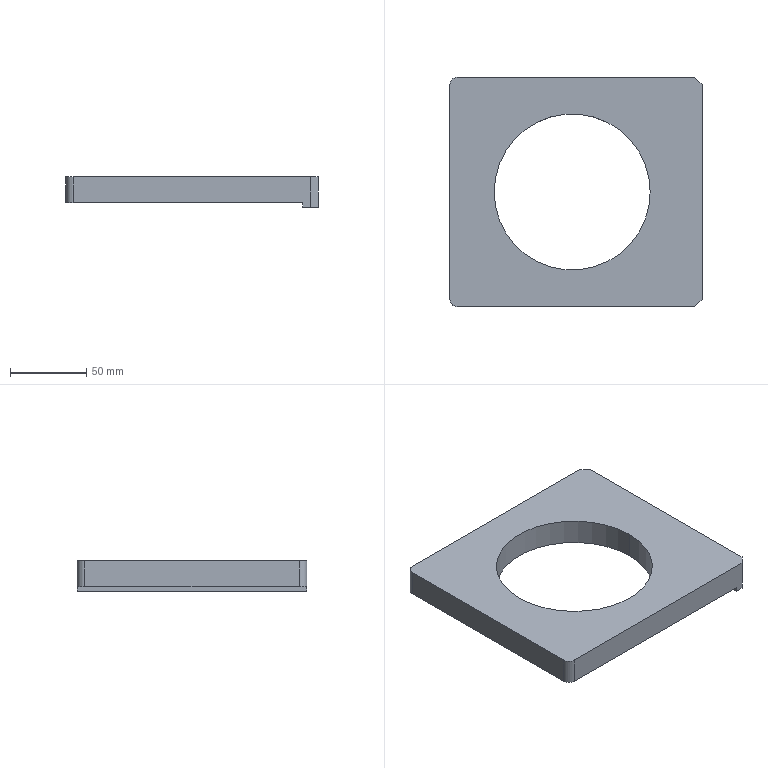Part | SolidWorks | features BaseBody 1 | 1 solid | 14 faces | box 165 x 150 x 20 mm | volume 285656 mm3 | plane 10 | cylinder 4 | commonest cylinder face diameters 10 x2 102 x2
STEP:
#1=CARTESIAN_POINT('',(-51.,0.,20.));
#2=VERTEX_POINT('',#1);
#3=CARTESIAN_POINT('',(51.,0.,20.));
#4=VERTEX_POINT('',#3);
#5=CARTESIAN_POINT('',(0.,0.,20.));
#6=DIRECTION('',(0.,0.,1.));
#7=DIRECTION('',(1.,0.,0.));
#8=AXIS2_PLACEMENT_3D('',#5,#6,#7);
#9=CIRCLE('',#8,51.);
#10=EDGE_CURVE('',#2,#4,#9,.T.);
#11=ORIENTED_EDGE('',*,*,#10,.T.);
#12=CARTESIAN_POINT('',(51.,0.,3.));
#13=VERTEX_POINT('',#12);
#14=CARTESIAN_POINT('',(51.,0.,20.));
#15=DIRECTION('',(0.,0.,-1.));
#16=VECTOR('',#15,1000.);
#17=LINE('',#14,#16);
#18=EDGE_CURVE('',#4,#13,#17,.T.);
#19=ORIENTED_EDGE('',*,*,#18,.T.);
#20=CARTESIAN_POINT('',(-51.,0.,3.));
#21=VERTEX_POINT('',#20);
#22=CARTESIAN_POINT('',(0.,0.,3.));
#23=DIRECTION('',(0.,0.,-1.));
#24=DIRECTION('',(-1.,0.,0.));
#25=AXIS2_PLACEMENT_3D('',#22,#23,#24);
#26=CIRCLE('',#25,51.);
#27=EDGE_CURVE('',#13,#21,#26,.T.);
#28=ORIENTED_EDGE('',*,*,#27,.T.);
#29=CARTESIAN_POINT('',(-51.,0.,20.));
#30=DIRECTION('',(0.,0.,-1.));
#31=VECTOR('',#30,1000.);
#32=LINE('',#29,#31);
#33=EDGE_CURVE('',#2,#21,#32,.T.);
#34=ORIENTED_EDGE('',*,*,#33,.F.);
#35=EDGE_LOOP('',(#11,#19,#28,#34));
#36=FACE_OUTER_BOUND('',#35,.T.);
#37=CARTESIAN_POINT('',(0.,0.,20.));
#38=DIRECTION('',(0.,0.,-1.));
#39=DIRECTION('',(-1.,0.,0.));
#40=AXIS2_PLACEMENT_3D('',#37,#38,#39);
#41=CYLINDRICAL_SURFACE('',#40,51.);
#42=ADVANCED_FACE('',(#36),#41,.F.);
#43=ORIENTED_EDGE('',*,*,#10,.F.);
#44=CARTESIAN_POINT('',(0.,0.,20.));
#45=DIRECTION('',(0.,0.,1.));
#46=DIRECTION('',(1.,0.,0.));
#47=AXIS2_PLACEMENT_3D('',#44,#45,#46);
#48=CIRCLE('',#47,51.);
#49=EDGE_CURVE('',#4,#2,#48,.T.);
#50=ORIENTED_EDGE('',*,*,#49,.F.);
#51=EDGE_LOOP('',(#43,#50));
#52=FACE_BOUND('',#51,.T.);
#53=CARTESIAN_POINT('',(-80.,-70.,20.));
#54=VERTEX_POINT('',#53);
#55=CARTESIAN_POINT('',(-75.,-75.,20.));
#56=VERTEX_POINT('',#55);
#57=CARTESIAN_POINT('',(-75.,-70.,20.));
#58=DIRECTION('',(0.,0.,1.));
#59=DIRECTION('',(1.,0.,0.));
#60=AXIS2_PLACEMENT_3D('',#57,#58,#59);
#61=CIRCLE('',#60,5.);
#62=EDGE_CURVE('',#54,#56,#61,.T.);
#63=ORIENTED_EDGE('',*,*,#62,.T.);
#64=CARTESIAN_POINT('',(80.,-75.,20.));
#65=VERTEX_POINT('',#64);
#66=CARTESIAN_POINT('',(0.,-75.,20.));
#67=DIRECTION('',(1.,0.,0.));
#68=VECTOR('',#67,1000.);
#69=LINE('',#66,#68);
#70=EDGE_CURVE('',#56,#65,#69,.T.);
#71=ORIENTED_EDGE('',*,*,#70,.T.);
#72=CARTESIAN_POINT('',(85.,-70.,20.));
#73=VERTEX_POINT('',#72);
#74=CARTESIAN_POINT('',(77.5,-77.5,20.));
#75=DIRECTION('',(0.7071,0.7071,0.));
#76=VECTOR('',#75,1000.);
#77=LINE('',#74,#76);
#78=EDGE_CURVE('',#65,#73,#77,.T.);
#79=ORIENTED_EDGE('',*,*,#78,.T.);
#80=CARTESIAN_POINT('',(85.,70.,20.));
#81=VERTEX_POINT('',#80);
#82=CARTESIAN_POINT('',(85.,80.,20.));
#83=DIRECTION('',(0.,1.,0.));
#84=VECTOR('',#83,1000.);
#85=LINE('',#82,#84);
#86=EDGE_CURVE('',#73,#81,#85,.T.);
#87=ORIENTED_EDGE('',*,*,#86,.T.);
#88=CARTESIAN_POINT('',(80.,75.,20.));
#89=VERTEX_POINT('',#88);
#90=CARTESIAN_POINT('',(77.5,77.5,20.));
#91=DIRECTION('',(-0.7071,0.7071,0.));
#92=VECTOR('',#91,1000.);
#93=LINE('',#90,#92);
#94=EDGE_CURVE('',#81,#89,#93,.T.);
#95=ORIENTED_EDGE('',*,*,#94,.T.);
#96=CARTESIAN_POINT('',(-75.,75.,20.));
#97=VERTEX_POINT('',#96);
#98=CARTESIAN_POINT('',(0.,75.,20.));
#99=DIRECTION('',(-1.,0.,0.));
#100=VECTOR('',#99,1000.);
#101=LINE('',#98,#100);
#102=EDGE_CURVE('',#89,#97,#101,.T.);
#103=ORIENTED_EDGE('',*,*,#102,.T.);
#104=CARTESIAN_POINT('',(-80.,70.,20.));
#105=VERTEX_POINT('',#104);
#106=CARTESIAN_POINT('',(-75.,70.,20.));
#107=DIRECTION('',(0.,0.,1.));
#108=DIRECTION('',(1.,0.,0.));
#109=AXIS2_PLACEMENT_3D('',#106,#107,#108);
#110=CIRCLE('',#109,5.);
#111=EDGE_CURVE('',#97,#105,#110,.T.);
#112=ORIENTED_EDGE('',*,*,#111,.T.);
#113=CARTESIAN_POINT('',(-80.,0.,20.));
#114=DIRECTION('',(0.,-1.,0.));
#115=VECTOR('',#114,1000.);
#116=LINE('',#113,#115);
#117=EDGE_CURVE('',#105,#54,#116,.T.);
#118=ORIENTED_EDGE('',*,*,#117,.T.);
#119=EDGE_LOOP('',(#63,#71,#79,#87,#95,#103,#112,#118));
#120=FACE_OUTER_BOUND('',#119,.T.);
#121=CARTESIAN_POINT('',(0.,0.,20.));
#122=DIRECTION('',(0.,0.,1.));
#123=DIRECTION('',(1.,0.,0.));
#124=AXIS2_PLACEMENT_3D('',#121,#122,#123);
#125=PLANE('',#124);
#126=ADVANCED_FACE('',(#52,#120),#125,.T.);
#127=CARTESIAN_POINT('',(75.,-75.,0.));
#128=VERTEX_POINT('',#127);
#129=CARTESIAN_POINT('',(80.,-75.,0.));
#130=VERTEX_POINT('',#129);
#131=CARTESIAN_POINT('',(0.,-75.,0.));
#132=DIRECTION('',(1.,0.,0.));
#133=VECTOR('',#132,1000.);
#134=LINE('',#131,#133);
#135=EDGE_CURVE('',#128,#130,#134,.T.);
#136=ORIENTED_EDGE('',*,*,#135,.F.);
#137=CARTESIAN_POINT('',(75.,75.,0.));
#138=VERTEX_POINT('',#137);
#139=CARTESIAN_POINT('',(75.,-80.,0.));
#140=DIRECTION('',(0.,-1.,0.));
#141=VECTOR('',#140,1000.);
#142=LINE('',#139,#141);
#143=EDGE_CURVE('',#138,#128,#142,.T.);
#144=ORIENTED_EDGE('',*,*,#143,.F.);
#145=CARTESIAN_POINT('',(80.,75.,0.));
#146=VERTEX_POINT('',#145);
#147=CARTESIAN_POINT('',(0.,75.,0.));
#148=DIRECTION('',(-1.,0.,0.));
#149=VECTOR('',#148,1000.);
#150=LINE('',#147,#149);
#151=EDGE_CURVE('',#146,#138,#150,.T.);
#152=ORIENTED_EDGE('',*,*,#151,.F.);
#153=CARTESIAN_POINT('',(85.,70.,0.));
#154=VERTEX_POINT('',#153);
#155=CARTESIAN_POINT('',(75.,80.,0.));
#156=DIRECTION('',(0.7071,-0.7071,0.));
#157=VECTOR('',#156,1000.);
#158=LINE('',#155,#157);
#159=EDGE_CURVE('',#146,#154,#158,.T.);
#160=ORIENTED_EDGE('',*,*,#159,.T.);
#161=CARTESIAN_POINT('',(85.,-70.,0.));
#162=VERTEX_POINT('',#161);
#163=CARTESIAN_POINT('',(85.,80.,0.));
#164=DIRECTION('',(0.,1.,0.));
#165=VECTOR('',#164,1000.);
#166=LINE('',#163,#165);
#167=EDGE_CURVE('',#162,#154,#166,.T.);
#168=ORIENTED_EDGE('',*,*,#167,.F.);
#169=CARTESIAN_POINT('',(85.,-70.,0.));
#170=DIRECTION('',(-0.7071,-0.7071,0.));
#171=VECTOR('',#170,1000.);
#172=LINE('',#169,#171);
#173=EDGE_CURVE('',#162,#130,#172,.T.);
#174=ORIENTED_EDGE('',*,*,#173,.T.);
#175=EDGE_LOOP('',(#136,#144,#152,#160,#168,#174));
#176=FACE_OUTER_BOUND('',#175,.T.);
#177=CARTESIAN_POINT('',(0.,0.,0.));
#178=DIRECTION('',(0.,0.,1.));
#179=DIRECTION('',(1.,0.,0.));
#180=AXIS2_PLACEMENT_3D('',#177,#178,#179);
#181=PLANE('',#180);
#182=ADVANCED_FACE('',(#176),#181,.F.);
#183=ORIENTED_EDGE('',*,*,#78,.F.);
#184=CARTESIAN_POINT('',(80.,-75.,20.));
#185=DIRECTION('',(0.,0.,-1.));
#186=VECTOR('',#185,1000.);
#187=LINE('',#184,#186);
#188=EDGE_CURVE('',#65,#130,#187,.T.);
#189=ORIENTED_EDGE('',*,*,#188,.T.);
#190=ORIENTED_EDGE('',*,*,#173,.F.);
#191=CARTESIAN_POINT('',(85.,-70.,20.));
#192=DIRECTION('',(0.,0.,-1.));
#193=VECTOR('',#192,1000.);
#194=LINE('',#191,#193);
#195=EDGE_CURVE('',#73,#162,#194,.T.);
#196=ORIENTED_EDGE('',*,*,#195,.F.);
#197=EDGE_LOOP('',(#183,#189,#190,#196));
#198=FACE_OUTER_BOUND('',#197,.T.);
#199=CARTESIAN_POINT('',(85.,-70.,20.));
#200=DIRECTION('',(-0.7071,0.7071,0.));
#201=DIRECTION('',(0.,0.,-1.));
#202=AXIS2_PLACEMENT_3D('',#199,#200,#201);
#203=PLANE('',#202);
#204=ADVANCED_FACE('',(#198),#203,.F.);
#205=ORIENTED_EDGE('',*,*,#159,.F.);
#206=CARTESIAN_POINT('',(80.,75.,20.));
#207=DIRECTION('',(0.,0.,1.));
#208=VECTOR('',#207,1000.);
#209=LINE('',#206,#208);
#210=EDGE_CURVE('',#146,#89,#209,.T.);
#211=ORIENTED_EDGE('',*,*,#210,.T.);
#212=ORIENTED_EDGE('',*,*,#94,.F.);
#213=CARTESIAN_POINT('',(85.,70.,20.));
#214=DIRECTION('',(0.,0.,1.));
#215=VECTOR('',#214,1000.);
#216=LINE('',#213,#215);
#217=EDGE_CURVE('',#154,#81,#216,.T.);
#218=ORIENTED_EDGE('',*,*,#217,.F.);
#219=EDGE_LOOP('',(#205,#211,#212,#218));
#220=FACE_OUTER_BOUND('',#219,.T.);
#221=CARTESIAN_POINT('',(75.,80.,20.));
#222=DIRECTION('',(-0.7071,-0.7071,0.));
#223=DIRECTION('',(0.,0.,-1.));
#224=AXIS2_PLACEMENT_3D('',#221,#222,#223);
#225=PLANE('',#224);
#226=ADVANCED_FACE('',(#220),#225,.F.);
#227=CARTESIAN_POINT('',(75.,-75.,3.));
#228=VERTEX_POINT('',#227);
#229=CARTESIAN_POINT('',(75.,-75.,3.));
#230=DIRECTION('',(0.,0.,-1.));
#231=VECTOR('',#230,1000.);
#232=LINE('',#229,#231);
#233=EDGE_CURVE('',#228,#128,#232,.T.);
#234=ORIENTED_EDGE('',*,*,#233,.F.);
#235=CARTESIAN_POINT('',(75.,75.,3.));
#236=VERTEX_POINT('',#235);
#237=CARTESIAN_POINT('',(75.,-80.,3.));
#238=DIRECTION('',(0.,-1.,0.));
#239=VECTOR('',#238,1000.);
#240=LINE('',#237,#239);
#241=EDGE_CURVE('',#236,#228,#240,.T.);
#242=ORIENTED_EDGE('',*,*,#241,.F.);
#243=CARTESIAN_POINT('',(75.,75.,3.));
#244=DIRECTION('',(0.,0.,1.));
#245=VECTOR('',#244,1000.);
#246=LINE('',#243,#245);
#247=EDGE_CURVE('',#138,#236,#246,.T.);
#248=ORIENTED_EDGE('',*,*,#247,.F.);
#249=ORIENTED_EDGE('',*,*,#143,.T.);
#250=EDGE_LOOP('',(#234,#242,#248,#249));
#251=FACE_OUTER_BOUND('',#250,.T.);
#252=CARTESIAN_POINT('',(75.,-80.,3.));
#253=DIRECTION('',(1.,0.,0.));
#254=DIRECTION('',(0.,0.,1.));
#255=AXIS2_PLACEMENT_3D('',#252,#253,#254);
#256=PLANE('',#255);
#257=ADVANCED_FACE('',(#251),#256,.F.);
#258=CARTESIAN_POINT('',(0.,0.,3.));
#259=DIRECTION('',(0.,0.,-1.));
#260=DIRECTION('',(-1.,0.,0.));
#261=AXIS2_PLACEMENT_3D('',#258,#259,#260);
#262=CIRCLE('',#261,51.);
#263=EDGE_CURVE('',#21,#13,#262,.T.);
#264=ORIENTED_EDGE('',*,*,#263,.F.);
#265=ORIENTED_EDGE('',*,*,#27,.F.);
#266=EDGE_LOOP('',(#264,#265));
#267=FACE_BOUND('',#266,.T.);
#268=ORIENTED_EDGE('',*,*,#241,.T.);
#269=CARTESIAN_POINT('',(-75.,-75.,3.));
#270=VERTEX_POINT('',#269);
#271=CARTESIAN_POINT('',(685.,-75.,3.));
#272=DIRECTION('',(-1.,0.,0.));
#273=VECTOR('',#272,1000.);
#274=LINE('',#271,#273);
#275=EDGE_CURVE('',#228,#270,#274,.T.);
#276=ORIENTED_EDGE('',*,*,#275,.T.);
#277=CARTESIAN_POINT('',(-80.,-70.,3.));
#278=VERTEX_POINT('',#277);
#279=CARTESIAN_POINT('',(-75.,-70.,3.));
#280=DIRECTION('',(0.,0.,-1.));
#281=DIRECTION('',(-1.,0.,0.));
#282=AXIS2_PLACEMENT_3D('',#279,#280,#281);
#283=CIRCLE('',#282,5.);
#284=EDGE_CURVE('',#270,#278,#283,.T.);
#285=ORIENTED_EDGE('',*,*,#284,.T.);
#286=CARTESIAN_POINT('',(-80.,70.,3.));
#287=VERTEX_POINT('',#286);
#288=CARTESIAN_POINT('',(-80.,0.,3.));
#289=DIRECTION('',(0.,1.,0.));
#290=VECTOR('',#289,1000.);
#291=LINE('',#288,#290);
#292=EDGE_CURVE('',#278,#287,#291,.T.);
#293=ORIENTED_EDGE('',*,*,#292,.T.);
#294=CARTESIAN_POINT('',(-75.,75.,3.));
#295=VERTEX_POINT('',#294);
#296=CARTESIAN_POINT('',(-75.,70.,3.));
#297=DIRECTION('',(0.,0.,-1.));
#298=DIRECTION('',(-1.,0.,0.));
#299=AXIS2_PLACEMENT_3D('',#296,#297,#298);
#300=CIRCLE('',#299,5.);
#301=EDGE_CURVE('',#287,#295,#300,.T.);
#302=ORIENTED_EDGE('',*,*,#301,.T.);
#303=CARTESIAN_POINT('',(685.,75.,3.));
#304=DIRECTION('',(1.,0.,0.));
#305=VECTOR('',#304,1000.);
#306=LINE('',#303,#305);
#307=EDGE_CURVE('',#295,#236,#306,.T.);
#308=ORIENTED_EDGE('',*,*,#307,.T.);
#309=EDGE_LOOP('',(#268,#276,#285,#293,#302,#308));
#310=FACE_OUTER_BOUND('',#309,.T.);
#311=CARTESIAN_POINT('',(685.,0.,3.));
#312=DIRECTION('',(0.,0.,-1.));
#313=DIRECTION('',(0.,1.,0.));
#314=AXIS2_PLACEMENT_3D('',#311,#312,#313);
#315=PLANE('',#314);
#316=ADVANCED_FACE('',(#267,#310),#315,.T.);
#317=ORIENTED_EDGE('',*,*,#18,.F.);
#318=ORIENTED_EDGE('',*,*,#49,.T.);
#319=ORIENTED_EDGE('',*,*,#33,.T.);
#320=ORIENTED_EDGE('',*,*,#263,.T.);
#321=EDGE_LOOP('',(#317,#318,#319,#320));
#322=FACE_OUTER_BOUND('',#321,.T.);
#323=CARTESIAN_POINT('',(0.,0.,20.));
#324=DIRECTION('',(0.,0.,-1.));
#325=DIRECTION('',(-1.,0.,0.));
#326=AXIS2_PLACEMENT_3D('',#323,#324,#325);
#327=CYLINDRICAL_SURFACE('',#326,51.);
#328=ADVANCED_FACE('',(#322),#327,.F.);
#329=ORIENTED_EDGE('',*,*,#86,.F.);
#330=ORIENTED_EDGE('',*,*,#195,.T.);
#331=ORIENTED_EDGE('',*,*,#167,.T.);
#332=ORIENTED_EDGE('',*,*,#217,.T.);
#333=EDGE_LOOP('',(#329,#330,#331,#332));
#334=FACE_OUTER_BOUND('',#333,.T.);
#335=CARTESIAN_POINT('',(85.,80.,20.));
#336=DIRECTION('',(-1.,0.,0.));
#337=DIRECTION('',(0.,-1.,0.));
#338=AXIS2_PLACEMENT_3D('',#335,#336,#337);
#339=PLANE('',#338);
#340=ADVANCED_FACE('',(#334),#339,.F.);
#341=CARTESIAN_POINT('',(-75.,-75.,-2.));
#342=DIRECTION('',(0.,0.,1.));
#343=VECTOR('',#342,1000.);
#344=LINE('',#341,#343);
#345=EDGE_CURVE('',#270,#56,#344,.T.);
#346=ORIENTED_EDGE('',*,*,#345,.F.);
#347=ORIENTED_EDGE('',*,*,#275,.F.);
#348=ORIENTED_EDGE('',*,*,#233,.T.);
#349=ORIENTED_EDGE('',*,*,#135,.T.);
#350=ORIENTED_EDGE('',*,*,#188,.F.);
#351=ORIENTED_EDGE('',*,*,#70,.F.);
#352=EDGE_LOOP('',(#346,#347,#348,#349,#350,#351));
#353=FACE_OUTER_BOUND('',#352,.T.);
#354=CARTESIAN_POINT('',(-75.,-75.,-2.));
#355=DIRECTION('',(0.,-1.,0.));
#356=DIRECTION('',(1.,0.,0.));
#357=AXIS2_PLACEMENT_3D('',#354,#355,#356);
#358=PLANE('',#357);
#359=ADVANCED_FACE('',(#353),#358,.T.);
#360=CARTESIAN_POINT('',(-80.,-70.,-2.));
#361=DIRECTION('',(0.,0.,1.));
#362=VECTOR('',#361,1000.);
#363=LINE('',#360,#362);
#364=EDGE_CURVE('',#278,#54,#363,.T.);
#365=ORIENTED_EDGE('',*,*,#364,.F.);
#366=ORIENTED_EDGE('',*,*,#284,.F.);
#367=ORIENTED_EDGE('',*,*,#345,.T.);
#368=ORIENTED_EDGE('',*,*,#62,.F.);
#369=EDGE_LOOP('',(#365,#366,#367,#368));
#370=FACE_OUTER_BOUND('',#369,.T.);
#371=CARTESIAN_POINT('',(-75.,-70.,-2.));
#372=DIRECTION('',(0.,0.,1.));
#373=DIRECTION('',(0.,-1.,0.));
#374=AXIS2_PLACEMENT_3D('',#371,#372,#373);
#375=CYLINDRICAL_SURFACE('',#374,5.);
#376=ADVANCED_FACE('',(#370),#375,.T.);
#377=CARTESIAN_POINT('',(-80.,70.,-2.));
#378=DIRECTION('',(0.,0.,1.));
#379=VECTOR('',#378,1000.);
#380=LINE('',#377,#379);
#381=EDGE_CURVE('',#287,#105,#380,.T.);
#382=ORIENTED_EDGE('',*,*,#381,.F.);
#383=ORIENTED_EDGE('',*,*,#292,.F.);
#384=ORIENTED_EDGE('',*,*,#364,.T.);
#385=ORIENTED_EDGE('',*,*,#117,.F.);
#386=EDGE_LOOP('',(#382,#383,#384,#385));
#387=FACE_OUTER_BOUND('',#386,.T.);
#388=CARTESIAN_POINT('',(-80.,70.,-2.));
#389=DIRECTION('',(-1.,0.,0.));
#390=DIRECTION('',(0.,-1.,0.));
#391=AXIS2_PLACEMENT_3D('',#388,#389,#390);
#392=PLANE('',#391);
#393=ADVANCED_FACE('',(#387),#392,.T.);
#394=CARTESIAN_POINT('',(-75.,75.,-2.));
#395=DIRECTION('',(0.,0.,1.));
#396=VECTOR('',#395,1000.);
#397=LINE('',#394,#396);
#398=EDGE_CURVE('',#295,#97,#397,.T.);
#399=ORIENTED_EDGE('',*,*,#398,.F.);
#400=ORIENTED_EDGE('',*,*,#301,.F.);
#401=ORIENTED_EDGE('',*,*,#381,.T.);
#402=ORIENTED_EDGE('',*,*,#111,.F.);
#403=EDGE_LOOP('',(#399,#400,#401,#402));
#404=FACE_OUTER_BOUND('',#403,.T.);
#405=CARTESIAN_POINT('',(-75.,70.,-2.));
#406=DIRECTION('',(0.,0.,1.));
#407=DIRECTION('',(0.,-1.,0.));
#408=AXIS2_PLACEMENT_3D('',#405,#406,#407);
#409=CYLINDRICAL_SURFACE('',#408,5.);
#410=ADVANCED_FACE('',(#404),#409,.T.);
#411=ORIENTED_EDGE('',*,*,#210,.F.);
#412=ORIENTED_EDGE('',*,*,#151,.T.);
#413=ORIENTED_EDGE('',*,*,#247,.T.);
#414=ORIENTED_EDGE('',*,*,#307,.F.);
#415=ORIENTED_EDGE('',*,*,#398,.T.);
#416=ORIENTED_EDGE('',*,*,#102,.F.);
#417=EDGE_LOOP('',(#411,#412,#413,#414,#415,#416));
#418=FACE_OUTER_BOUND('',#417,.T.);
#419=CARTESIAN_POINT('',(-75.,75.,-2.));
#420=DIRECTION('',(0.,1.,0.));
#421=DIRECTION('',(-1.,0.,0.));
#422=AXIS2_PLACEMENT_3D('',#419,#420,#421);
#423=PLANE('',#422);
#424=ADVANCED_FACE('',(#418),#423,.T.);
#425=CLOSED_SHELL('',(#42,#126,#182,#204,#226,#257,#316,#328,#340,#359,#376,#393,#410,#424));
#426=MANIFOLD_SOLID_BREP('',#425);
#427=CARTESIAN_POINT('',(0.,0.,0.));
#428=DIRECTION('',(0.,0.,1.));
#429=DIRECTION('',(1.,0.,0.));
#430=AXIS2_PLACEMENT_3D('',#427,#428,#429);
#431=(LENGTH_UNIT()NAMED_UNIT(*)SI_UNIT(.MILLI.,.METRE.));
#432=UNCERTAINTY_MEASURE_WITH_UNIT(LENGTH_MEASURE(0.00001),#431,'','');
#433=(NAMED_UNIT(*)PLANE_ANGLE_UNIT()SI_UNIT($,.RADIAN.));
#434=(NAMED_UNIT(*)SI_UNIT($,.STERADIAN.)SOLID_ANGLE_UNIT());
#435=(GEOMETRIC_REPRESENTATION_CONTEXT(3)GLOBAL_UNCERTAINTY_ASSIGNED_CONTEXT((#432))GLOBAL_UNIT_ASSIGNED_CONTEXT((#431,#433,#434))REPRESENTATION_CONTEXT('',''));
#436=ADVANCED_BREP_SHAPE_REPRESENTATION('',(#426,#430),#435);